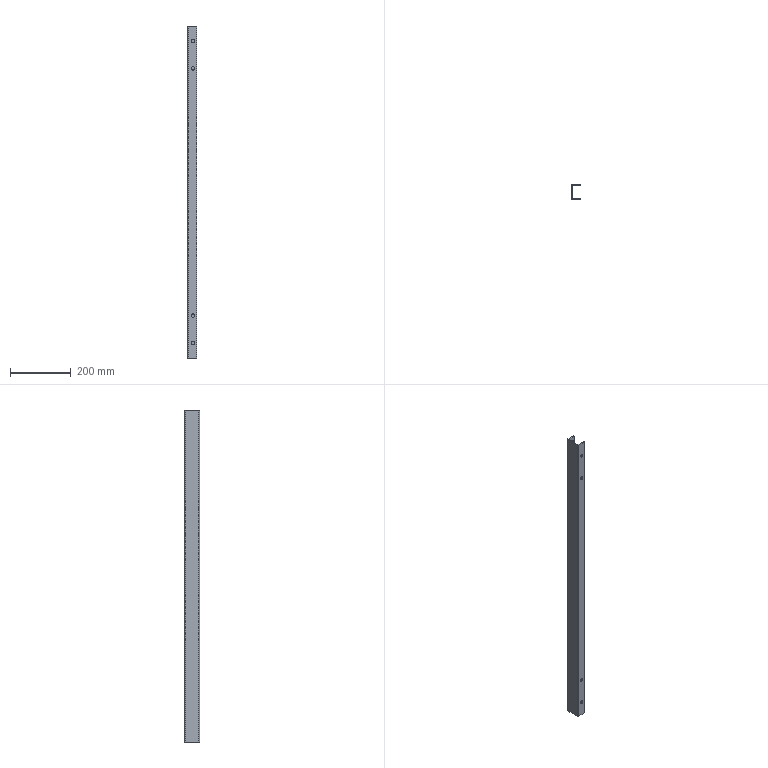Part | 1 solid | 55 faces | box 30 x 50 x 1096 mm | volume 331835 mm3 | plane 28 | cylinder 27 | commonest cylinder face diameters 10 x15 11 x8 0.4 x2 6.4 x2